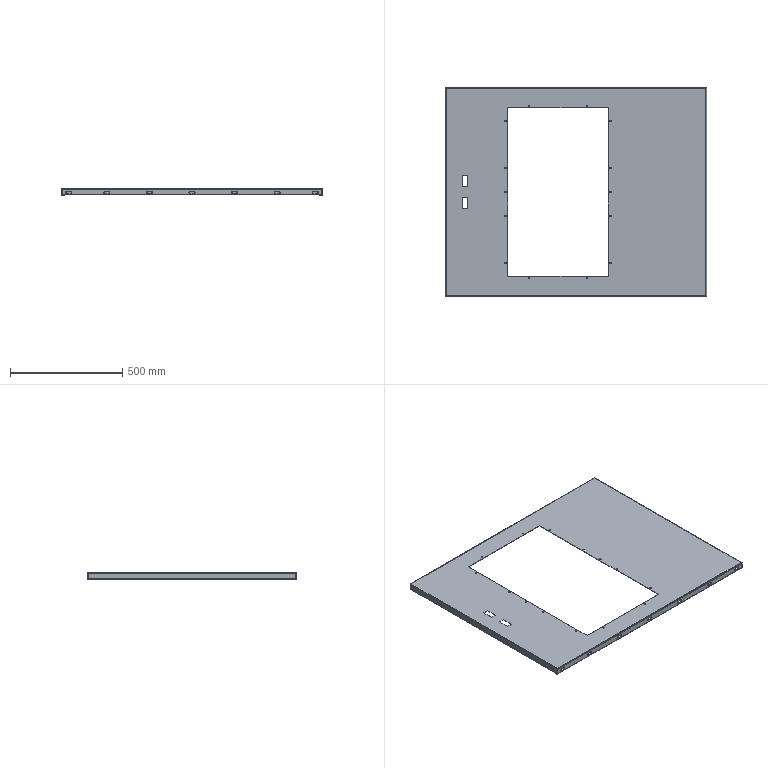Part | SolidWorks | features BaseBody 1 | 1 solid | 222 faces | box 1165 x 930 x 30 mm | volume 1834786 mm3 | plane 144 | cylinder 78 | commonest cylinder face diameters 6 x37 10 x14 12 x14 2 x9 0.1 x2 4.1 x2